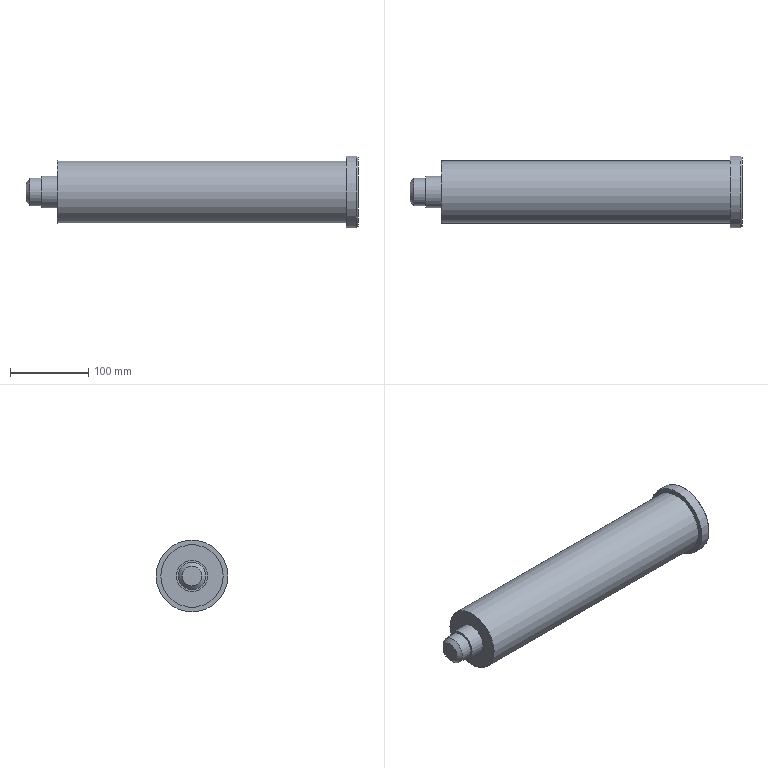Part | NX | features solid 2 | 1 solid | 11 faces | box 425 x 92 x 92 mm | volume 2002099 mm3 | plane 5 | cylinder 4 | cone 2 | commonest cylinder face diameters 35 x1 40 x1 80 x1 92 x1
STEP:
#1=CARTESIAN_POINT('',(1854.,-1250.,-480.));
#2=VERTEX_POINT('',#1);
#3=CARTESIAN_POINT('',(1854.,-1210.,-480.));
#4=DIRECTION('',(-1.,0.,0.));
#5=DIRECTION('',(0.,-1.,0.));
#6=AXIS2_PLACEMENT_3D('',#3,#4,#5);
#7=CIRCLE('',#6,40.);
#8=EDGE_CURVE('',#2,#2,#7,.T.);
#9=ORIENTED_EDGE('',*,*,#8,.F.);
#10=EDGE_LOOP('',(#9));
#11=FACE_BOUND('',#10,.T.);
#12=CARTESIAN_POINT('',(2224.,-1250.,-480.));
#13=VERTEX_POINT('',#12);
#14=CARTESIAN_POINT('',(2224.,-1210.,-480.));
#15=DIRECTION('',(-1.,0.,0.));
#16=DIRECTION('',(0.,-1.,0.));
#17=AXIS2_PLACEMENT_3D('',#14,#15,#16);
#18=CIRCLE('',#17,40.);
#19=EDGE_CURVE('',#13,#13,#18,.T.);
#20=ORIENTED_EDGE('',*,*,#19,.T.);
#21=EDGE_LOOP('',(#20));
#22=FACE_BOUND('',#21,.T.);
#23=CARTESIAN_POINT('',(1854.,-1210.,-480.));
#24=DIRECTION('',(1.,0.,0.));
#25=DIRECTION('',(0.,-1.,0.));
#26=AXIS2_PLACEMENT_3D('',#23,#24,#25);
#27=CYLINDRICAL_SURFACE('',#26,40.);
#28=ADVANCED_FACE('',(#11,#22),#27,.T.);
#29=CARTESIAN_POINT('',(1854.,-1230.,-480.));
#30=VERTEX_POINT('',#29);
#31=CARTESIAN_POINT('',(1854.,-1210.,-480.));
#32=DIRECTION('',(-1.,0.,0.));
#33=DIRECTION('',(0.,-1.,0.));
#34=AXIS2_PLACEMENT_3D('',#31,#32,#33);
#35=CIRCLE('',#34,20.);
#36=EDGE_CURVE('',#30,#30,#35,.T.);
#37=ORIENTED_EDGE('',*,*,#36,.F.);
#38=EDGE_LOOP('',(#37));
#39=FACE_BOUND('',#38,.T.);
#40=ORIENTED_EDGE('',*,*,#8,.T.);
#41=EDGE_LOOP('',(#40));
#42=FACE_BOUND('',#41,.T.);
#43=CARTESIAN_POINT('',(1854.,-1210.,-480.));
#44=DIRECTION('',(1.,0.,0.));
#45=DIRECTION('',(0.,-1.,0.));
#46=AXIS2_PLACEMENT_3D('',#43,#44,#45);
#47=PLANE('',#46);
#48=ADVANCED_FACE('',(#39,#42),#47,.F.);
#49=CARTESIAN_POINT('',(2237.,-1256.,-480.));
#50=VERTEX_POINT('',#49);
#51=CARTESIAN_POINT('',(2237.,-1210.,-480.));
#52=DIRECTION('',(-1.,0.,0.));
#53=DIRECTION('',(0.,-1.,0.));
#54=AXIS2_PLACEMENT_3D('',#51,#52,#53);
#55=CIRCLE('',#54,46.);
#56=EDGE_CURVE('',#50,#50,#55,.F.);
#57=ORIENTED_EDGE('',*,*,#56,.F.);
#58=EDGE_LOOP('',(#57));
#59=FACE_BOUND('',#58,.T.);
#60=CARTESIAN_POINT('',(2224.,-1256.,-480.));
#61=VERTEX_POINT('',#60);
#62=CARTESIAN_POINT('',(2224.,-1210.,-480.));
#63=DIRECTION('',(-1.,0.,0.));
#64=DIRECTION('',(0.,-1.,0.));
#65=AXIS2_PLACEMENT_3D('',#62,#63,#64);
#66=CIRCLE('',#65,46.);
#67=EDGE_CURVE('',#61,#61,#66,.T.);
#68=ORIENTED_EDGE('',*,*,#67,.F.);
#69=EDGE_LOOP('',(#68));
#70=FACE_BOUND('',#69,.T.);
#71=CARTESIAN_POINT('',(2224.,-1210.,-480.));
#72=DIRECTION('',(1.,0.,0.));
#73=DIRECTION('',(0.,-1.,0.));
#74=AXIS2_PLACEMENT_3D('',#71,#72,#73);
#75=CYLINDRICAL_SURFACE('',#74,46.);
#76=ADVANCED_FACE('',(#59,#70),#75,.T.);
#77=ORIENTED_EDGE('',*,*,#19,.F.);
#78=EDGE_LOOP('',(#77));
#79=FACE_BOUND('',#78,.T.);
#80=ORIENTED_EDGE('',*,*,#67,.T.);
#81=EDGE_LOOP('',(#80));
#82=FACE_BOUND('',#81,.T.);
#83=CARTESIAN_POINT('',(2224.,-1210.,-480.));
#84=DIRECTION('',(1.,0.,0.));
#85=DIRECTION('',(0.,-1.,0.));
#86=AXIS2_PLACEMENT_3D('',#83,#84,#85);
#87=PLANE('',#86);
#88=ADVANCED_FACE('',(#79,#82),#87,.F.);
#89=CARTESIAN_POINT('',(2239.,-1254.,-480.));
#90=VERTEX_POINT('',#89);
#91=CARTESIAN_POINT('',(2239.,-1210.,-480.));
#92=DIRECTION('',(-1.,0.,0.));
#93=DIRECTION('',(0.,-1.,0.));
#94=AXIS2_PLACEMENT_3D('',#91,#92,#93);
#95=CIRCLE('',#94,44.);
#96=EDGE_CURVE('',#90,#90,#95,.T.);
#97=ORIENTED_EDGE('',*,*,#96,.F.);
#98=EDGE_LOOP('',(#97));
#99=FACE_BOUND('',#98,.T.);
#100=CARTESIAN_POINT('',(2239.,-1210.,-480.));
#101=DIRECTION('',(1.,0.,0.));
#102=DIRECTION('',(0.,-1.,0.));
#103=AXIS2_PLACEMENT_3D('',#100,#101,#102);
#104=PLANE('',#103);
#105=ADVANCED_FACE('',(#99),#104,.T.);
#106=CARTESIAN_POINT('',(1834.,-1230.,-480.));
#107=VERTEX_POINT('',#106);
#108=CARTESIAN_POINT('',(1834.,-1210.,-480.));
#109=DIRECTION('',(-1.,0.,0.));
#110=DIRECTION('',(0.,-1.,0.));
#111=AXIS2_PLACEMENT_3D('',#108,#109,#110);
#112=CIRCLE('',#111,20.);
#113=EDGE_CURVE('',#107,#107,#112,.T.);
#114=ORIENTED_EDGE('',*,*,#113,.F.);
#115=EDGE_LOOP('',(#114));
#116=FACE_BOUND('',#115,.T.);
#117=ORIENTED_EDGE('',*,*,#36,.T.);
#118=EDGE_LOOP('',(#117));
#119=FACE_BOUND('',#118,.T.);
#120=CARTESIAN_POINT('',(1834.,-1210.,-480.));
#121=DIRECTION('',(1.,0.,0.));
#122=DIRECTION('',(0.,-1.,0.));
#123=AXIS2_PLACEMENT_3D('',#120,#121,#122);
#124=CYLINDRICAL_SURFACE('',#123,20.);
#125=ADVANCED_FACE('',(#116,#119),#124,.T.);
#126=CARTESIAN_POINT('',(1834.,-1227.5,-480.));
#127=VERTEX_POINT('',#126);
#128=CARTESIAN_POINT('',(1834.,-1210.,-480.));
#129=DIRECTION('',(-1.,0.,0.));
#130=DIRECTION('',(0.,-1.,0.));
#131=AXIS2_PLACEMENT_3D('',#128,#129,#130);
#132=CIRCLE('',#131,17.5);
#133=EDGE_CURVE('',#127,#127,#132,.T.);
#134=ORIENTED_EDGE('',*,*,#133,.F.);
#135=EDGE_LOOP('',(#134));
#136=FACE_BOUND('',#135,.T.);
#137=ORIENTED_EDGE('',*,*,#113,.T.);
#138=EDGE_LOOP('',(#137));
#139=FACE_BOUND('',#138,.T.);
#140=CARTESIAN_POINT('',(1834.,-1210.,-480.));
#141=DIRECTION('',(1.,0.,0.));
#142=DIRECTION('',(0.,-1.,0.));
#143=AXIS2_PLACEMENT_3D('',#140,#141,#142);
#144=PLANE('',#143);
#145=ADVANCED_FACE('',(#136,#139),#144,.F.);
#146=CARTESIAN_POINT('',(1819.,-1227.5,-480.));
#147=VERTEX_POINT('',#146);
#148=CARTESIAN_POINT('',(1819.,-1210.,-480.));
#149=DIRECTION('',(-1.,0.,0.));
#150=DIRECTION('',(0.,-1.,0.));
#151=AXIS2_PLACEMENT_3D('',#148,#149,#150);
#152=CIRCLE('',#151,17.5);
#153=EDGE_CURVE('',#147,#147,#152,.T.);
#154=ORIENTED_EDGE('',*,*,#153,.F.);
#155=EDGE_LOOP('',(#154));
#156=FACE_BOUND('',#155,.T.);
#157=ORIENTED_EDGE('',*,*,#133,.T.);
#158=EDGE_LOOP('',(#157));
#159=FACE_BOUND('',#158,.T.);
#160=CARTESIAN_POINT('',(1814.,-1210.,-480.));
#161=DIRECTION('',(1.,0.,0.));
#162=DIRECTION('',(0.,-1.,0.));
#163=AXIS2_PLACEMENT_3D('',#160,#161,#162);
#164=CYLINDRICAL_SURFACE('',#163,17.5);
#165=ADVANCED_FACE('',(#156,#159),#164,.T.);
#166=CARTESIAN_POINT('',(1814.,-1222.5,-480.));
#167=VERTEX_POINT('',#166);
#168=CARTESIAN_POINT('',(1814.,-1210.,-480.));
#169=DIRECTION('',(-1.,0.,0.));
#170=DIRECTION('',(0.,-1.,0.));
#171=AXIS2_PLACEMENT_3D('',#168,#169,#170);
#172=CIRCLE('',#171,12.5);
#173=EDGE_CURVE('',#167,#167,#172,.F.);
#174=ORIENTED_EDGE('',*,*,#173,.F.);
#175=EDGE_LOOP('',(#174));
#176=FACE_BOUND('',#175,.T.);
#177=CARTESIAN_POINT('',(1814.,-1210.,-480.));
#178=DIRECTION('',(1.,0.,0.));
#179=DIRECTION('',(0.,-1.,0.));
#180=AXIS2_PLACEMENT_3D('',#177,#178,#179);
#181=PLANE('',#180);
#182=ADVANCED_FACE('',(#176),#181,.F.);
#183=ORIENTED_EDGE('',*,*,#173,.T.);
#184=EDGE_LOOP('',(#183));
#185=FACE_BOUND('',#184,.T.);
#186=ORIENTED_EDGE('',*,*,#153,.T.);
#187=EDGE_LOOP('',(#186));
#188=FACE_BOUND('',#187,.T.);
#189=CARTESIAN_POINT('',(1819.,-1210.,-480.));
#190=DIRECTION('',(1.,0.,0.));
#191=DIRECTION('',(0.,-1.,0.));
#192=AXIS2_PLACEMENT_3D('',#189,#190,#191);
#193=CONICAL_SURFACE('',#192,17.5,0.7854);
#194=ADVANCED_FACE('',(#185,#188),#193,.T.);
#195=ORIENTED_EDGE('',*,*,#56,.T.);
#196=EDGE_LOOP('',(#195));
#197=FACE_BOUND('',#196,.T.);
#198=ORIENTED_EDGE('',*,*,#96,.T.);
#199=EDGE_LOOP('',(#198));
#200=FACE_BOUND('',#199,.T.);
#201=CARTESIAN_POINT('',(2239.,-1210.,-480.));
#202=DIRECTION('',(-1.,0.,0.));
#203=DIRECTION('',(0.,1.,0.));
#204=AXIS2_PLACEMENT_3D('',#201,#202,#203);
#205=CONICAL_SURFACE('',#204,44.,0.7854);
#206=ADVANCED_FACE('',(#197,#200),#205,.T.);
#207=CLOSED_SHELL('',(#28,#48,#76,#88,#105,#125,#145,#165,#182,#194,#206));
#208=MANIFOLD_SOLID_BREP('',#207);
#209=(LENGTH_UNIT()NAMED_UNIT(*)SI_UNIT(.MILLI.,.METRE.));
#210=UNCERTAINTY_MEASURE_WITH_UNIT(LENGTH_MEASURE(0.00001),#209,'','');
#211=(NAMED_UNIT(*)PLANE_ANGLE_UNIT()SI_UNIT($,.RADIAN.));
#212=(NAMED_UNIT(*)SI_UNIT($,.STERADIAN.)SOLID_ANGLE_UNIT());
#213=(GEOMETRIC_REPRESENTATION_CONTEXT(3)GLOBAL_UNCERTAINTY_ASSIGNED_CONTEXT((#210))GLOBAL_UNIT_ASSIGNED_CONTEXT((#209,#211,#212))REPRESENTATION_CONTEXT('',''));
#214=ADVANCED_BREP_SHAPE_REPRESENTATION('',(#208),#213);